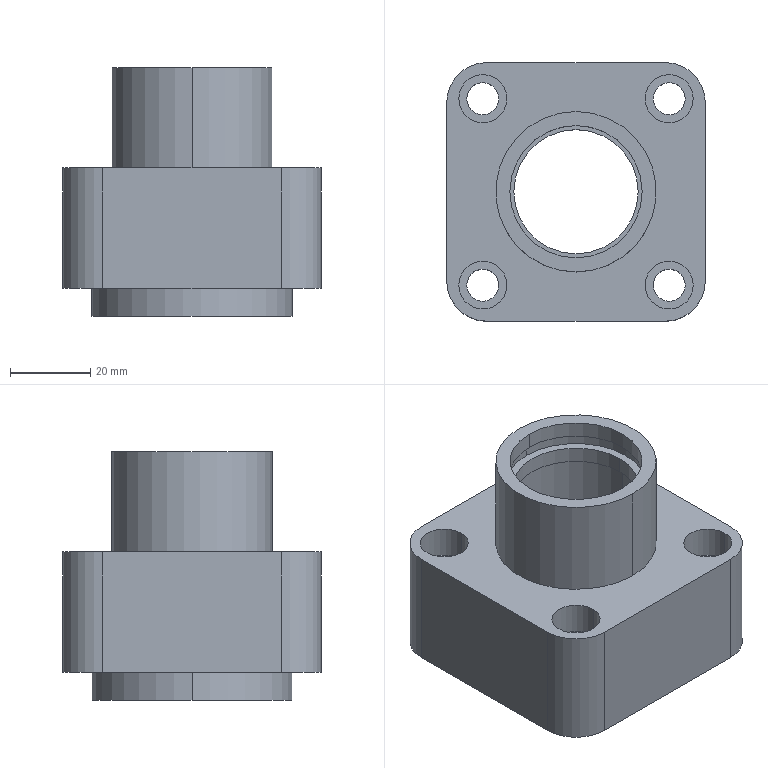Part | STEP file | 1 solid | 52 faces | box 64.5 x 64.5 x 62 mm | volume 97512 mm3 | cylinder 36 | plane 16 | commonest cylinder face diameters 8 x8 12 x8 20 x4 33 x4 40 x4 6.917 x2